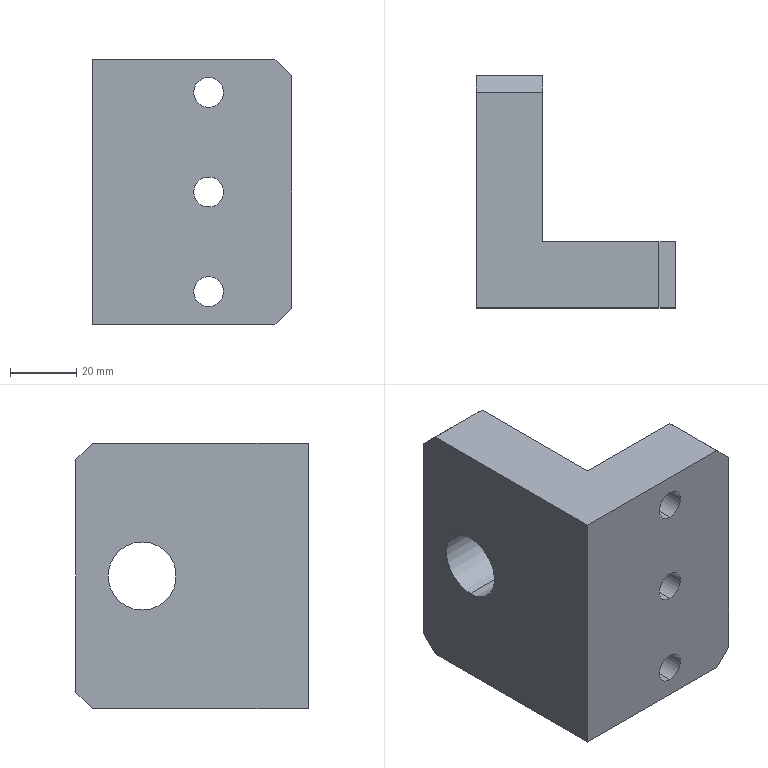Part | SolidWorks | features BaseBody 1 | 1 solid | 29 faces | box 60 x 70 x 80 mm | volume 161528 mm3 | plane 15 | cylinder 14 | commonest cylinder face diameters 9 x6 15 x6 20.5 x2
STEP:
#1=CARTESIAN_POINT('',(0.,50.,50.25));
#2=VERTEX_POINT('',#1);
#3=CARTESIAN_POINT('',(0.,50.,29.75));
#4=VERTEX_POINT('',#3);
#5=CARTESIAN_POINT('',(0.,50.,40.));
#6=DIRECTION('',(1.,0.,0.));
#7=DIRECTION('',(0.,0.,-1.));
#8=AXIS2_PLACEMENT_3D('',#5,#6,#7);
#9=CIRCLE('',#8,10.25);
#10=EDGE_CURVE('',#2,#4,#9,.T.);
#11=ORIENTED_EDGE('',*,*,#10,.F.);
#12=CARTESIAN_POINT('',(20.,50.,50.25));
#13=VERTEX_POINT('',#12);
#14=CARTESIAN_POINT('',(20.,50.,50.25));
#15=DIRECTION('',(1.,0.,0.));
#16=VECTOR('',#15,1000.);
#17=LINE('',#14,#16);
#18=EDGE_CURVE('',#2,#13,#17,.T.);
#19=ORIENTED_EDGE('',*,*,#18,.T.);
#20=CARTESIAN_POINT('',(20.,50.,29.75));
#21=VERTEX_POINT('',#20);
#22=CARTESIAN_POINT('',(20.,50.,40.));
#23=DIRECTION('',(1.,0.,0.));
#24=DIRECTION('',(0.,0.,-1.));
#25=AXIS2_PLACEMENT_3D('',#22,#23,#24);
#26=CIRCLE('',#25,10.25);
#27=EDGE_CURVE('',#13,#21,#26,.T.);
#28=ORIENTED_EDGE('',*,*,#27,.T.);
#29=CARTESIAN_POINT('',(20.,50.,29.75));
#30=DIRECTION('',(1.,0.,0.));
#31=VECTOR('',#30,1000.);
#32=LINE('',#29,#31);
#33=EDGE_CURVE('',#4,#21,#32,.T.);
#34=ORIENTED_EDGE('',*,*,#33,.F.);
#35=EDGE_LOOP('',(#11,#19,#28,#34));
#36=FACE_OUTER_BOUND('',#35,.T.);
#37=CARTESIAN_POINT('',(20.,50.,40.));
#38=DIRECTION('',(1.,0.,0.));
#39=DIRECTION('',(0.,0.,-1.));
#40=AXIS2_PLACEMENT_3D('',#37,#38,#39);
#41=CYLINDRICAL_SURFACE('',#40,10.25);
#42=ADVANCED_FACE('',(#36),#41,.F.);
#43=CARTESIAN_POINT('',(35.,11.,2.5));
#44=VERTEX_POINT('',#43);
#45=CARTESIAN_POINT('',(35.,11.,17.5));
#46=VERTEX_POINT('',#45);
#47=CARTESIAN_POINT('',(35.,11.,10.));
#48=DIRECTION('',(0.,1.,0.));
#49=DIRECTION('',(0.,0.,1.));
#50=AXIS2_PLACEMENT_3D('',#47,#48,#49);
#51=CIRCLE('',#50,7.5);
#52=EDGE_CURVE('',#44,#46,#51,.T.);
#53=ORIENTED_EDGE('',*,*,#52,.F.);
#54=CARTESIAN_POINT('',(35.,20.,2.5));
#55=VERTEX_POINT('',#54);
#56=CARTESIAN_POINT('',(35.,20.,2.5));
#57=DIRECTION('',(0.,1.,0.));
#58=VECTOR('',#57,1000.);
#59=LINE('',#56,#58);
#60=EDGE_CURVE('',#44,#55,#59,.T.);
#61=ORIENTED_EDGE('',*,*,#60,.T.);
#62=CARTESIAN_POINT('',(35.,20.,17.5));
#63=VERTEX_POINT('',#62);
#64=CARTESIAN_POINT('',(35.,20.,10.));
#65=DIRECTION('',(0.,1.,0.));
#66=DIRECTION('',(0.,0.,1.));
#67=AXIS2_PLACEMENT_3D('',#64,#65,#66);
#68=CIRCLE('',#67,7.5);
#69=EDGE_CURVE('',#55,#63,#68,.T.);
#70=ORIENTED_EDGE('',*,*,#69,.T.);
#71=CARTESIAN_POINT('',(35.,20.,17.5));
#72=DIRECTION('',(0.,1.,0.));
#73=VECTOR('',#72,1000.);
#74=LINE('',#71,#73);
#75=EDGE_CURVE('',#46,#63,#74,.T.);
#76=ORIENTED_EDGE('',*,*,#75,.F.);
#77=EDGE_LOOP('',(#53,#61,#70,#76));
#78=FACE_OUTER_BOUND('',#77,.T.);
#79=CARTESIAN_POINT('',(35.,20.,10.));
#80=DIRECTION('',(0.,1.,0.));
#81=DIRECTION('',(0.,0.,1.));
#82=AXIS2_PLACEMENT_3D('',#79,#80,#81);
#83=CYLINDRICAL_SURFACE('',#82,7.5);
#84=ADVANCED_FACE('',(#78),#83,.F.);
#85=CARTESIAN_POINT('',(35.,0.,5.5));
#86=VERTEX_POINT('',#85);
#87=CARTESIAN_POINT('',(35.,0.,14.5));
#88=VERTEX_POINT('',#87);
#89=CARTESIAN_POINT('',(35.,0.,10.));
#90=DIRECTION('',(0.,1.,0.));
#91=DIRECTION('',(0.,0.,1.));
#92=AXIS2_PLACEMENT_3D('',#89,#90,#91);
#93=CIRCLE('',#92,4.5);
#94=EDGE_CURVE('',#86,#88,#93,.T.);
#95=ORIENTED_EDGE('',*,*,#94,.F.);
#96=CARTESIAN_POINT('',(35.,11.,5.5));
#97=VERTEX_POINT('',#96);
#98=CARTESIAN_POINT('',(35.,20.,5.5));
#99=DIRECTION('',(0.,1.,0.));
#100=VECTOR('',#99,1000.);
#101=LINE('',#98,#100);
#102=EDGE_CURVE('',#86,#97,#101,.T.);
#103=ORIENTED_EDGE('',*,*,#102,.T.);
#104=CARTESIAN_POINT('',(35.,11.,14.5));
#105=VERTEX_POINT('',#104);
#106=CARTESIAN_POINT('',(35.,11.,10.));
#107=DIRECTION('',(0.,1.,0.));
#108=DIRECTION('',(0.,0.,1.));
#109=AXIS2_PLACEMENT_3D('',#106,#107,#108);
#110=CIRCLE('',#109,4.5);
#111=EDGE_CURVE('',#97,#105,#110,.T.);
#112=ORIENTED_EDGE('',*,*,#111,.T.);
#113=CARTESIAN_POINT('',(35.,20.,14.5));
#114=DIRECTION('',(0.,1.,0.));
#115=VECTOR('',#114,1000.);
#116=LINE('',#113,#115);
#117=EDGE_CURVE('',#88,#105,#116,.T.);
#118=ORIENTED_EDGE('',*,*,#117,.F.);
#119=EDGE_LOOP('',(#95,#103,#112,#118));
#120=FACE_OUTER_BOUND('',#119,.T.);
#121=CARTESIAN_POINT('',(35.,20.,10.));
#122=DIRECTION('',(0.,1.,0.));
#123=DIRECTION('',(0.,0.,1.));
#124=AXIS2_PLACEMENT_3D('',#121,#122,#123);
#125=CYLINDRICAL_SURFACE('',#124,4.5);
#126=ADVANCED_FACE('',(#120),#125,.F.);
#127=CARTESIAN_POINT('',(35.,11.,32.5));
#128=VERTEX_POINT('',#127);
#129=CARTESIAN_POINT('',(35.,11.,47.5));
#130=VERTEX_POINT('',#129);
#131=CARTESIAN_POINT('',(35.,11.,40.));
#132=DIRECTION('',(0.,1.,0.));
#133=DIRECTION('',(0.,0.,1.));
#134=AXIS2_PLACEMENT_3D('',#131,#132,#133);
#135=CIRCLE('',#134,7.5);
#136=EDGE_CURVE('',#128,#130,#135,.T.);
#137=ORIENTED_EDGE('',*,*,#136,.F.);
#138=CARTESIAN_POINT('',(35.,20.,32.5));
#139=VERTEX_POINT('',#138);
#140=CARTESIAN_POINT('',(35.,20.,32.5));
#141=DIRECTION('',(0.,1.,0.));
#142=VECTOR('',#141,1000.);
#143=LINE('',#140,#142);
#144=EDGE_CURVE('',#128,#139,#143,.T.);
#145=ORIENTED_EDGE('',*,*,#144,.T.);
#146=CARTESIAN_POINT('',(35.,20.,47.5));
#147=VERTEX_POINT('',#146);
#148=CARTESIAN_POINT('',(35.,20.,40.));
#149=DIRECTION('',(0.,1.,0.));
#150=DIRECTION('',(0.,0.,1.));
#151=AXIS2_PLACEMENT_3D('',#148,#149,#150);
#152=CIRCLE('',#151,7.5);
#153=EDGE_CURVE('',#139,#147,#152,.T.);
#154=ORIENTED_EDGE('',*,*,#153,.T.);
#155=CARTESIAN_POINT('',(35.,20.,47.5));
#156=DIRECTION('',(0.,1.,0.));
#157=VECTOR('',#156,1000.);
#158=LINE('',#155,#157);
#159=EDGE_CURVE('',#130,#147,#158,.T.);
#160=ORIENTED_EDGE('',*,*,#159,.F.);
#161=EDGE_LOOP('',(#137,#145,#154,#160));
#162=FACE_OUTER_BOUND('',#161,.T.);
#163=CARTESIAN_POINT('',(35.,20.,40.));
#164=DIRECTION('',(0.,1.,0.));
#165=DIRECTION('',(0.,0.,1.));
#166=AXIS2_PLACEMENT_3D('',#163,#164,#165);
#167=CYLINDRICAL_SURFACE('',#166,7.5);
#168=ADVANCED_FACE('',(#162),#167,.F.);
#169=CARTESIAN_POINT('',(35.,0.,35.5));
#170=VERTEX_POINT('',#169);
#171=CARTESIAN_POINT('',(35.,0.,44.5));
#172=VERTEX_POINT('',#171);
#173=CARTESIAN_POINT('',(35.,0.,40.));
#174=DIRECTION('',(0.,1.,0.));
#175=DIRECTION('',(0.,0.,1.));
#176=AXIS2_PLACEMENT_3D('',#173,#174,#175);
#177=CIRCLE('',#176,4.5);
#178=EDGE_CURVE('',#170,#172,#177,.T.);
#179=ORIENTED_EDGE('',*,*,#178,.F.);
#180=CARTESIAN_POINT('',(35.,11.,35.5));
#181=VERTEX_POINT('',#180);
#182=CARTESIAN_POINT('',(35.,20.,35.5));
#183=DIRECTION('',(0.,1.,0.));
#184=VECTOR('',#183,1000.);
#185=LINE('',#182,#184);
#186=EDGE_CURVE('',#170,#181,#185,.T.);
#187=ORIENTED_EDGE('',*,*,#186,.T.);
#188=CARTESIAN_POINT('',(35.,11.,44.5));
#189=VERTEX_POINT('',#188);
#190=CARTESIAN_POINT('',(35.,11.,40.));
#191=DIRECTION('',(0.,1.,0.));
#192=DIRECTION('',(0.,0.,1.));
#193=AXIS2_PLACEMENT_3D('',#190,#191,#192);
#194=CIRCLE('',#193,4.5);
#195=EDGE_CURVE('',#181,#189,#194,.T.);
#196=ORIENTED_EDGE('',*,*,#195,.T.);
#197=CARTESIAN_POINT('',(35.,20.,44.5));
#198=DIRECTION('',(0.,1.,0.));
#199=VECTOR('',#198,1000.);
#200=LINE('',#197,#199);
#201=EDGE_CURVE('',#172,#189,#200,.T.);
#202=ORIENTED_EDGE('',*,*,#201,.F.);
#203=EDGE_LOOP('',(#179,#187,#196,#202));
#204=FACE_OUTER_BOUND('',#203,.T.);
#205=CARTESIAN_POINT('',(35.,20.,40.));
#206=DIRECTION('',(0.,1.,0.));
#207=DIRECTION('',(0.,0.,1.));
#208=AXIS2_PLACEMENT_3D('',#205,#206,#207);
#209=CYLINDRICAL_SURFACE('',#208,4.5);
#210=ADVANCED_FACE('',(#204),#209,.F.);
#211=CARTESIAN_POINT('',(35.,11.,62.5));
#212=VERTEX_POINT('',#211);
#213=CARTESIAN_POINT('',(35.,11.,77.5));
#214=VERTEX_POINT('',#213);
#215=CARTESIAN_POINT('',(35.,11.,70.));
#216=DIRECTION('',(0.,1.,0.));
#217=DIRECTION('',(0.,0.,1.));
#218=AXIS2_PLACEMENT_3D('',#215,#216,#217);
#219=CIRCLE('',#218,7.5);
#220=EDGE_CURVE('',#212,#214,#219,.T.);
#221=ORIENTED_EDGE('',*,*,#220,.F.);
#222=CARTESIAN_POINT('',(35.,20.,62.5));
#223=VERTEX_POINT('',#222);
#224=CARTESIAN_POINT('',(35.,20.,62.5));
#225=DIRECTION('',(0.,1.,0.));
#226=VECTOR('',#225,1000.);
#227=LINE('',#224,#226);
#228=EDGE_CURVE('',#212,#223,#227,.T.);
#229=ORIENTED_EDGE('',*,*,#228,.T.);
#230=CARTESIAN_POINT('',(35.,20.,77.5));
#231=VERTEX_POINT('',#230);
#232=CARTESIAN_POINT('',(35.,20.,70.));
#233=DIRECTION('',(0.,1.,0.));
#234=DIRECTION('',(0.,0.,1.));
#235=AXIS2_PLACEMENT_3D('',#232,#233,#234);
#236=CIRCLE('',#235,7.5);
#237=EDGE_CURVE('',#223,#231,#236,.T.);
#238=ORIENTED_EDGE('',*,*,#237,.T.);
#239=CARTESIAN_POINT('',(35.,20.,77.5));
#240=DIRECTION('',(0.,1.,0.));
#241=VECTOR('',#240,1000.);
#242=LINE('',#239,#241);
#243=EDGE_CURVE('',#214,#231,#242,.T.);
#244=ORIENTED_EDGE('',*,*,#243,.F.);
#245=EDGE_LOOP('',(#221,#229,#238,#244));
#246=FACE_OUTER_BOUND('',#245,.T.);
#247=CARTESIAN_POINT('',(35.,20.,70.));
#248=DIRECTION('',(0.,1.,0.));
#249=DIRECTION('',(0.,0.,1.));
#250=AXIS2_PLACEMENT_3D('',#247,#248,#249);
#251=CYLINDRICAL_SURFACE('',#250,7.5);
#252=ADVANCED_FACE('',(#246),#251,.F.);
#253=CARTESIAN_POINT('',(35.,0.,65.5));
#254=VERTEX_POINT('',#253);
#255=CARTESIAN_POINT('',(35.,0.,74.5));
#256=VERTEX_POINT('',#255);
#257=CARTESIAN_POINT('',(35.,0.,70.));
#258=DIRECTION('',(0.,1.,0.));
#259=DIRECTION('',(0.,0.,1.));
#260=AXIS2_PLACEMENT_3D('',#257,#258,#259);
#261=CIRCLE('',#260,4.5);
#262=EDGE_CURVE('',#254,#256,#261,.T.);
#263=ORIENTED_EDGE('',*,*,#262,.F.);
#264=CARTESIAN_POINT('',(35.,11.,65.5));
#265=VERTEX_POINT('',#264);
#266=CARTESIAN_POINT('',(35.,20.,65.5));
#267=DIRECTION('',(0.,1.,0.));
#268=VECTOR('',#267,1000.);
#269=LINE('',#266,#268);
#270=EDGE_CURVE('',#254,#265,#269,.T.);
#271=ORIENTED_EDGE('',*,*,#270,.T.);
#272=CARTESIAN_POINT('',(35.,11.,74.5));
#273=VERTEX_POINT('',#272);
#274=CARTESIAN_POINT('',(35.,11.,70.));
#275=DIRECTION('',(0.,1.,0.));
#276=DIRECTION('',(0.,0.,1.));
#277=AXIS2_PLACEMENT_3D('',#274,#275,#276);
#278=CIRCLE('',#277,4.5);
#279=EDGE_CURVE('',#265,#273,#278,.T.);
#280=ORIENTED_EDGE('',*,*,#279,.T.);
#281=CARTESIAN_POINT('',(35.,20.,74.5));
#282=DIRECTION('',(0.,1.,0.));
#283=VECTOR('',#282,1000.);
#284=LINE('',#281,#283);
#285=EDGE_CURVE('',#256,#273,#284,.T.);
#286=ORIENTED_EDGE('',*,*,#285,.F.);
#287=EDGE_LOOP('',(#263,#271,#280,#286));
#288=FACE_OUTER_BOUND('',#287,.T.);
#289=CARTESIAN_POINT('',(35.,20.,70.));
#290=DIRECTION('',(0.,1.,0.));
#291=DIRECTION('',(0.,0.,1.));
#292=AXIS2_PLACEMENT_3D('',#289,#290,#291);
#293=CYLINDRICAL_SURFACE('',#292,4.5);
#294=ADVANCED_FACE('',(#288),#293,.F.);
#295=CARTESIAN_POINT('',(35.,0.,10.));
#296=DIRECTION('',(0.,1.,0.));
#297=DIRECTION('',(0.,0.,1.));
#298=AXIS2_PLACEMENT_3D('',#295,#296,#297);
#299=CIRCLE('',#298,4.5);
#300=EDGE_CURVE('',#88,#86,#299,.T.);
#301=ORIENTED_EDGE('',*,*,#300,.T.);
#302=ORIENTED_EDGE('',*,*,#94,.T.);
#303=EDGE_LOOP('',(#301,#302));
#304=FACE_BOUND('',#303,.T.);
#305=CARTESIAN_POINT('',(35.,0.,40.));
#306=DIRECTION('',(0.,1.,0.));
#307=DIRECTION('',(0.,0.,1.));
#308=AXIS2_PLACEMENT_3D('',#305,#306,#307);
#309=CIRCLE('',#308,4.5);
#310=EDGE_CURVE('',#172,#170,#309,.T.);
#311=ORIENTED_EDGE('',*,*,#310,.T.);
#312=ORIENTED_EDGE('',*,*,#178,.T.);
#313=EDGE_LOOP('',(#311,#312));
#314=FACE_BOUND('',#313,.T.);
#315=CARTESIAN_POINT('',(35.,0.,70.));
#316=DIRECTION('',(0.,1.,0.));
#317=DIRECTION('',(0.,0.,1.));
#318=AXIS2_PLACEMENT_3D('',#315,#316,#317);
#319=CIRCLE('',#318,4.5);
#320=EDGE_CURVE('',#256,#254,#319,.T.);
#321=ORIENTED_EDGE('',*,*,#320,.T.);
#322=ORIENTED_EDGE('',*,*,#262,.T.);
#323=EDGE_LOOP('',(#321,#322));
#324=FACE_BOUND('',#323,.T.);
#325=CARTESIAN_POINT('',(0.,0.,0.));
#326=VERTEX_POINT('',#325);
#327=CARTESIAN_POINT('',(55.,0.,0.));
#328=VERTEX_POINT('',#327);
#329=CARTESIAN_POINT('',(60.,0.,0.));
#330=DIRECTION('',(1.,0.,0.));
#331=VECTOR('',#330,1000.);
#332=LINE('',#329,#331);
#333=EDGE_CURVE('',#326,#328,#332,.T.);
#334=ORIENTED_EDGE('',*,*,#333,.T.);
#335=CARTESIAN_POINT('',(60.,0.,5.));
#336=VERTEX_POINT('',#335);
#337=CARTESIAN_POINT('',(60.,0.,5.));
#338=DIRECTION('',(0.7071,0.,0.7071));
#339=VECTOR('',#338,1000.);
#340=LINE('',#337,#339);
#341=EDGE_CURVE('',#328,#336,#340,.T.);
#342=ORIENTED_EDGE('',*,*,#341,.T.);
#343=CARTESIAN_POINT('',(60.,0.,75.));
#344=VERTEX_POINT('',#343);
#345=CARTESIAN_POINT('',(60.,0.,80.));
#346=DIRECTION('',(0.,0.,-1.));
#347=VECTOR('',#346,1000.);
#348=LINE('',#345,#347);
#349=EDGE_CURVE('',#344,#336,#348,.T.);
#350=ORIENTED_EDGE('',*,*,#349,.F.);
#351=CARTESIAN_POINT('',(55.,0.,80.));
#352=VERTEX_POINT('',#351);
#353=CARTESIAN_POINT('',(55.,0.,80.));
#354=DIRECTION('',(-0.7071,0.,0.7071));
#355=VECTOR('',#354,1000.);
#356=LINE('',#353,#355);
#357=EDGE_CURVE('',#344,#352,#356,.T.);
#358=ORIENTED_EDGE('',*,*,#357,.T.);
#359=CARTESIAN_POINT('',(0.,0.,80.));
#360=VERTEX_POINT('',#359);
#361=CARTESIAN_POINT('',(60.,0.,80.));
#362=DIRECTION('',(1.,0.,0.));
#363=VECTOR('',#362,1000.);
#364=LINE('',#361,#363);
#365=EDGE_CURVE('',#360,#352,#364,.T.);
#366=ORIENTED_EDGE('',*,*,#365,.F.);
#367=CARTESIAN_POINT('',(0.,0.,80.));
#368=DIRECTION('',(0.,0.,-1.));
#369=VECTOR('',#368,1000.);
#370=LINE('',#367,#369);
#371=EDGE_CURVE('',#360,#326,#370,.T.);
#372=ORIENTED_EDGE('',*,*,#371,.T.);
#373=EDGE_LOOP('',(#334,#342,#350,#358,#366,#372));
#374=FACE_OUTER_BOUND('',#373,.T.);
#375=CARTESIAN_POINT('',(60.,0.,80.));
#376=DIRECTION('',(0.,1.,0.));
#377=DIRECTION('',(-1.,0.,0.));
#378=AXIS2_PLACEMENT_3D('',#375,#376,#377);
#379=PLANE('',#378);
#380=ADVANCED_FACE('',(#304,#314,#324,#374),#379,.F.);
#381=ORIENTED_EDGE('',*,*,#349,.T.);
#382=CARTESIAN_POINT('',(60.,20.,5.));
#383=VERTEX_POINT('',#382);
#384=CARTESIAN_POINT('',(60.,20.,5.));
#385=DIRECTION('',(0.,1.,0.));
#386=VECTOR('',#385,1000.);
#387=LINE('',#384,#386);
#388=EDGE_CURVE('',#336,#383,#387,.T.);
#389=ORIENTED_EDGE('',*,*,#388,.T.);
#390=CARTESIAN_POINT('',(60.,20.,75.));
#391=VERTEX_POINT('',#390);
#392=CARTESIAN_POINT('',(60.,20.,80.));
#393=DIRECTION('',(0.,0.,-1.));
#394=VECTOR('',#393,1000.);
#395=LINE('',#392,#394);
#396=EDGE_CURVE('',#391,#383,#395,.T.);
#397=ORIENTED_EDGE('',*,*,#396,.F.);
#398=CARTESIAN_POINT('',(60.,20.,75.));
#399=DIRECTION('',(0.,-1.,0.));
#400=VECTOR('',#399,1000.);
#401=LINE('',#398,#400);
#402=EDGE_CURVE('',#391,#344,#401,.T.);
#403=ORIENTED_EDGE('',*,*,#402,.T.);
#404=EDGE_LOOP('',(#381,#389,#397,#403));
#405=FACE_OUTER_BOUND('',#404,.T.);
#406=CARTESIAN_POINT('',(60.,20.,80.));
#407=DIRECTION('',(-1.,0.,0.));
#408=DIRECTION('',(0.,0.,1.));
#409=AXIS2_PLACEMENT_3D('',#406,#407,#408);
#410=PLANE('',#409);
#411=ADVANCED_FACE('',(#405),#410,.F.);
#412=CARTESIAN_POINT('',(35.,20.,10.));
#413=DIRECTION('',(0.,1.,0.));
#414=DIRECTION('',(0.,0.,1.));
#415=AXIS2_PLACEMENT_3D('',#412,#413,#414);
#416=CIRCLE('',#415,7.5);
#417=EDGE_CURVE('',#63,#55,#416,.T.);
#418=ORIENTED_EDGE('',*,*,#417,.F.);
#419=ORIENTED_EDGE('',*,*,#69,.F.);
#420=EDGE_LOOP('',(#418,#419));
#421=FACE_BOUND('',#420,.T.);
#422=CARTESIAN_POINT('',(35.,20.,40.));
#423=DIRECTION('',(0.,1.,0.));
#424=DIRECTION('',(0.,0.,1.));
#425=AXIS2_PLACEMENT_3D('',#422,#423,#424);
#426=CIRCLE('',#425,7.5);
#427=EDGE_CURVE('',#147,#139,#426,.T.);
#428=ORIENTED_EDGE('',*,*,#427,.F.);
#429=ORIENTED_EDGE('',*,*,#153,.F.);
#430=EDGE_LOOP('',(#428,#429));
#431=FACE_BOUND('',#430,.T.);
#432=CARTESIAN_POINT('',(35.,20.,70.));
#433=DIRECTION('',(0.,1.,0.));
#434=DIRECTION('',(0.,0.,1.));
#435=AXIS2_PLACEMENT_3D('',#432,#433,#434);
#436=CIRCLE('',#435,7.5);
#437=EDGE_CURVE('',#231,#223,#436,.T.);
#438=ORIENTED_EDGE('',*,*,#437,.F.);
#439=ORIENTED_EDGE('',*,*,#237,.F.);
#440=EDGE_LOOP('',(#438,#439));
#441=FACE_BOUND('',#440,.T.);
#442=ORIENTED_EDGE('',*,*,#396,.T.);
#443=CARTESIAN_POINT('',(55.,20.,0.));
#444=VERTEX_POINT('',#443);
#445=CARTESIAN_POINT('',(60.,20.,5.));
#446=DIRECTION('',(-0.7071,0.,-0.7071));
#447=VECTOR('',#446,1000.);
#448=LINE('',#445,#447);
#449=EDGE_CURVE('',#383,#444,#448,.T.);
#450=ORIENTED_EDGE('',*,*,#449,.T.);
#451=CARTESIAN_POINT('',(20.,20.,0.));
#452=VERTEX_POINT('',#451);
#453=CARTESIAN_POINT('',(20.,20.,0.));
#454=DIRECTION('',(-1.,0.,0.));
#455=VECTOR('',#454,1000.);
#456=LINE('',#453,#455);
#457=EDGE_CURVE('',#444,#452,#456,.T.);
#458=ORIENTED_EDGE('',*,*,#457,.T.);
#459=CARTESIAN_POINT('',(20.,20.,80.));
#460=VERTEX_POINT('',#459);
#461=CARTESIAN_POINT('',(20.,20.,80.));
#462=DIRECTION('',(0.,0.,-1.));
#463=VECTOR('',#462,1000.);
#464=LINE('',#461,#463);
#465=EDGE_CURVE('',#460,#452,#464,.T.);
#466=ORIENTED_EDGE('',*,*,#465,.F.);
#467=CARTESIAN_POINT('',(55.,20.,80.));
#468=VERTEX_POINT('',#467);
#469=CARTESIAN_POINT('',(20.,20.,80.));
#470=DIRECTION('',(-1.,0.,0.));
#471=VECTOR('',#470,1000.);
#472=LINE('',#469,#471);
#473=EDGE_CURVE('',#468,#460,#472,.T.);
#474=ORIENTED_EDGE('',*,*,#473,.F.);
#475=CARTESIAN_POINT('',(55.,20.,80.));
#476=DIRECTION('',(0.7071,0.,-0.7071));
#477=VECTOR('',#476,1000.);
#478=LINE('',#475,#477);
#479=EDGE_CURVE('',#468,#391,#478,.T.);
#480=ORIENTED_EDGE('',*,*,#479,.T.);
#481=EDGE_LOOP('',(#442,#450,#458,#466,#474,#480));
#482=FACE_OUTER_BOUND('',#481,.T.);
#483=CARTESIAN_POINT('',(20.,20.,80.));
#484=DIRECTION('',(0.,-1.,0.));
#485=DIRECTION('',(0.,0.,-1.));
#486=AXIS2_PLACEMENT_3D('',#483,#484,#485);
#487=PLANE('',#486);
#488=ADVANCED_FACE('',(#421,#431,#441,#482),#487,.F.);
#489=CARTESIAN_POINT('',(20.,50.,40.));
#490=DIRECTION('',(1.,0.,0.));
#491=DIRECTION('',(0.,0.,-1.));
#492=AXIS2_PLACEMENT_3D('',#489,#490,#491);
#493=CIRCLE('',#492,10.25);
#494=EDGE_CURVE('',#21,#13,#493,.T.);
#495=ORIENTED_EDGE('',*,*,#494,.F.);
#496=ORIENTED_EDGE('',*,*,#27,.F.);
#497=EDGE_LOOP('',(#495,#496));
#498=FACE_BOUND('',#497,.T.);
#499=CARTESIAN_POINT('',(20.,70.,75.));
#500=VERTEX_POINT('',#499);
#501=CARTESIAN_POINT('',(20.,70.,5.));
#502=VERTEX_POINT('',#501);
#503=CARTESIAN_POINT('',(20.,70.,80.));
#504=DIRECTION('',(0.,0.,-1.));
#505=VECTOR('',#504,1000.);
#506=LINE('',#503,#505);
#507=EDGE_CURVE('',#500,#502,#506,.T.);
#508=ORIENTED_EDGE('',*,*,#507,.F.);
#509=CARTESIAN_POINT('',(20.,65.,80.));
#510=VERTEX_POINT('',#509);
#511=CARTESIAN_POINT('',(20.,65.,80.));
#512=DIRECTION('',(0.,-0.7071,0.7071));
#513=VECTOR('',#512,1000.);
#514=LINE('',#511,#513);
#515=EDGE_CURVE('',#500,#510,#514,.T.);
#516=ORIENTED_EDGE('',*,*,#515,.T.);
#517=CARTESIAN_POINT('',(20.,70.,80.));
#518=DIRECTION('',(0.,1.,0.));
#519=VECTOR('',#518,1000.);
#520=LINE('',#517,#519);
#521=EDGE_CURVE('',#460,#510,#520,.T.);
#522=ORIENTED_EDGE('',*,*,#521,.F.);
#523=ORIENTED_EDGE('',*,*,#465,.T.);
#524=CARTESIAN_POINT('',(20.,65.,0.));
#525=VERTEX_POINT('',#524);
#526=CARTESIAN_POINT('',(20.,70.,0.));
#527=DIRECTION('',(0.,1.,0.));
#528=VECTOR('',#527,1000.);
#529=LINE('',#526,#528);
#530=EDGE_CURVE('',#452,#525,#529,.T.);
#531=ORIENTED_EDGE('',*,*,#530,.T.);
#532=CARTESIAN_POINT('',(20.,70.,5.));
#533=DIRECTION('',(0.,0.7071,0.7071));
#534=VECTOR('',#533,1000.);
#535=LINE('',#532,#534);
#536=EDGE_CURVE('',#525,#502,#535,.T.);
#537=ORIENTED_EDGE('',*,*,#536,.T.);
#538=EDGE_LOOP('',(#508,#516,#522,#523,#531,#537));
#539=FACE_OUTER_BOUND('',#538,.T.);
#540=CARTESIAN_POINT('',(20.,70.,80.));
#541=DIRECTION('',(-1.,0.,0.));
#542=DIRECTION('',(0.,-1.,0.));
#543=AXIS2_PLACEMENT_3D('',#540,#541,#542);
#544=PLANE('',#543);
#545=ADVANCED_FACE('',(#498,#539),#544,.F.);
#546=CARTESIAN_POINT('',(0.,70.,75.));
#547=VERTEX_POINT('',#546);
#548=CARTESIAN_POINT('',(0.,70.,5.));
#549=VERTEX_POINT('',#548);
#550=CARTESIAN_POINT('',(0.,70.,80.));
#551=DIRECTION('',(0.,0.,-1.));
#552=VECTOR('',#551,1000.);
#553=LINE('',#550,#552);
#554=EDGE_CURVE('',#547,#549,#553,.T.);
#555=ORIENTED_EDGE('',*,*,#554,.F.);
#556=CARTESIAN_POINT('',(0.,70.,75.));
#557=DIRECTION('',(1.,0.,0.));
#558=VECTOR('',#557,1000.);
#559=LINE('',#556,#558);
#560=EDGE_CURVE('',#547,#500,#559,.T.);
#561=ORIENTED_EDGE('',*,*,#560,.T.);
#562=ORIENTED_EDGE('',*,*,#507,.T.);
#563=CARTESIAN_POINT('',(0.,70.,5.));
#564=DIRECTION('',(-1.,0.,0.));
#565=VECTOR('',#564,1000.);
#566=LINE('',#563,#565);
#567=EDGE_CURVE('',#502,#549,#566,.T.);
#568=ORIENTED_EDGE('',*,*,#567,.T.);
#569=EDGE_LOOP('',(#555,#561,#562,#568));
#570=FACE_OUTER_BOUND('',#569,.T.);
#571=CARTESIAN_POINT('',(0.,70.,80.));
#572=DIRECTION('',(0.,-1.,0.));
#573=DIRECTION('',(0.,0.,-1.));
#574=AXIS2_PLACEMENT_3D('',#571,#572,#573);
#575=PLANE('',#574);
#576=ADVANCED_FACE('',(#570),#575,.F.);
#577=CARTESIAN_POINT('',(0.,50.,40.));
#578=DIRECTION('',(1.,0.,0.));
#579=DIRECTION('',(0.,0.,-1.));
#580=AXIS2_PLACEMENT_3D('',#577,#578,#579);
#581=CIRCLE('',#580,10.25);
#582=EDGE_CURVE('',#4,#2,#581,.T.);
#583=ORIENTED_EDGE('',*,*,#582,.T.);
#584=ORIENTED_EDGE('',*,*,#10,.T.);
#585=EDGE_LOOP('',(#583,#584));
#586=FACE_BOUND('',#585,.T.);
#587=CARTESIAN_POINT('',(0.,65.,80.));
#588=VERTEX_POINT('',#587);
#589=CARTESIAN_POINT('',(0.,0.,80.));
#590=DIRECTION('',(0.,-1.,0.));
#591=VECTOR('',#590,1000.);
#592=LINE('',#589,#591);
#593=EDGE_CURVE('',#588,#360,#592,.T.);
#594=ORIENTED_EDGE('',*,*,#593,.F.);
#595=CARTESIAN_POINT('',(0.,65.,80.));
#596=DIRECTION('',(0.,0.7071,-0.7071));
#597=VECTOR('',#596,1000.);
#598=LINE('',#595,#597);
#599=EDGE_CURVE('',#588,#547,#598,.T.);
#600=ORIENTED_EDGE('',*,*,#599,.T.);
#601=ORIENTED_EDGE('',*,*,#554,.T.);
#602=CARTESIAN_POINT('',(0.,65.,0.));
#603=VERTEX_POINT('',#602);
#604=CARTESIAN_POINT('',(0.,70.,5.));
#605=DIRECTION('',(0.,-0.7071,-0.7071));
#606=VECTOR('',#605,1000.);
#607=LINE('',#604,#606);
#608=EDGE_CURVE('',#549,#603,#607,.T.);
#609=ORIENTED_EDGE('',*,*,#608,.T.);
#610=CARTESIAN_POINT('',(0.,0.,0.));
#611=DIRECTION('',(0.,-1.,0.));
#612=VECTOR('',#611,1000.);
#613=LINE('',#610,#612);
#614=EDGE_CURVE('',#603,#326,#613,.T.);
#615=ORIENTED_EDGE('',*,*,#614,.T.);
#616=ORIENTED_EDGE('',*,*,#371,.F.);
#617=EDGE_LOOP('',(#594,#600,#601,#609,#615,#616));
#618=FACE_OUTER_BOUND('',#617,.T.);
#619=CARTESIAN_POINT('',(0.,0.,80.));
#620=DIRECTION('',(1.,0.,0.));
#621=DIRECTION('',(0.,0.,-1.));
#622=AXIS2_PLACEMENT_3D('',#619,#620,#621);
#623=PLANE('',#622);
#624=ADVANCED_FACE('',(#586,#618),#623,.F.);
#625=ORIENTED_EDGE('',*,*,#521,.T.);
#626=CARTESIAN_POINT('',(0.,65.,80.));
#627=DIRECTION('',(-1.,0.,0.));
#628=VECTOR('',#627,1000.);
#629=LINE('',#626,#628);
#630=EDGE_CURVE('',#510,#588,#629,.T.);
#631=ORIENTED_EDGE('',*,*,#630,.T.);
#632=ORIENTED_EDGE('',*,*,#593,.T.);
#633=ORIENTED_EDGE('',*,*,#365,.T.);
#634=CARTESIAN_POINT('',(55.,0.,80.));
#635=DIRECTION('',(0.,1.,0.));
#636=VECTOR('',#635,1000.);
#637=LINE('',#634,#636);
#638=EDGE_CURVE('',#352,#468,#637,.T.);
#639=ORIENTED_EDGE('',*,*,#638,.T.);
#640=ORIENTED_EDGE('',*,*,#473,.T.);
#641=EDGE_LOOP('',(#625,#631,#632,#633,#639,#640));
#642=FACE_OUTER_BOUND('',#641,.T.);
#643=CARTESIAN_POINT('',(0.,0.,80.));
#644=DIRECTION('',(0.,0.,-1.));
#645=DIRECTION('',(-1.,0.,0.));
#646=AXIS2_PLACEMENT_3D('',#643,#644,#645);
#647=PLANE('',#646);
#648=ADVANCED_FACE('',(#642),#647,.F.);
#649=ORIENTED_EDGE('',*,*,#614,.F.);
#650=CARTESIAN_POINT('',(20.,65.,0.));
#651=DIRECTION('',(1.,0.,0.));
#652=VECTOR('',#651,1000.);
#653=LINE('',#650,#652);
#654=EDGE_CURVE('',#603,#525,#653,.T.);
#655=ORIENTED_EDGE('',*,*,#654,.T.);
#656=ORIENTED_EDGE('',*,*,#530,.F.);
#657=ORIENTED_EDGE('',*,*,#457,.F.);
#658=CARTESIAN_POINT('',(55.,0.,0.));
#659=DIRECTION('',(0.,-1.,0.));
#660=VECTOR('',#659,1000.);
#661=LINE('',#658,#660);
#662=EDGE_CURVE('',#444,#328,#661,.T.);
#663=ORIENTED_EDGE('',*,*,#662,.T.);
#664=ORIENTED_EDGE('',*,*,#333,.F.);
#665=EDGE_LOOP('',(#649,#655,#656,#657,#663,#664));
#666=FACE_OUTER_BOUND('',#665,.T.);
#667=CARTESIAN_POINT('',(0.,0.,0.));
#668=DIRECTION('',(0.,0.,-1.));
#669=DIRECTION('',(-1.,0.,0.));
#670=AXIS2_PLACEMENT_3D('',#667,#668,#669);
#671=PLANE('',#670);
#672=ADVANCED_FACE('',(#666),#671,.T.);
#673=ORIENTED_EDGE('',*,*,#270,.F.);
#674=ORIENTED_EDGE('',*,*,#320,.F.);
#675=ORIENTED_EDGE('',*,*,#285,.T.);
#676=CARTESIAN_POINT('',(35.,11.,70.));
#677=DIRECTION('',(0.,1.,0.));
#678=DIRECTION('',(0.,0.,1.));
#679=AXIS2_PLACEMENT_3D('',#676,#677,#678);
#680=CIRCLE('',#679,4.5);
#681=EDGE_CURVE('',#273,#265,#680,.T.);
#682=ORIENTED_EDGE('',*,*,#681,.T.);
#683=EDGE_LOOP('',(#673,#674,#675,#682));
#684=FACE_OUTER_BOUND('',#683,.T.);
#685=CARTESIAN_POINT('',(35.,20.,70.));
#686=DIRECTION('',(0.,1.,0.));
#687=DIRECTION('',(0.,0.,1.));
#688=AXIS2_PLACEMENT_3D('',#685,#686,#687);
#689=CYLINDRICAL_SURFACE('',#688,4.5);
#690=ADVANCED_FACE('',(#684),#689,.F.);
#691=ORIENTED_EDGE('',*,*,#681,.F.);
#692=ORIENTED_EDGE('',*,*,#279,.F.);
#693=EDGE_LOOP('',(#691,#692));
#694=FACE_BOUND('',#693,.T.);
#695=CARTESIAN_POINT('',(35.,11.,70.));
#696=DIRECTION('',(0.,1.,0.));
#697=DIRECTION('',(0.,0.,1.));
#698=AXIS2_PLACEMENT_3D('',#695,#696,#697);
#699=CIRCLE('',#698,7.5);
#700=EDGE_CURVE('',#214,#212,#699,.T.);
#701=ORIENTED_EDGE('',*,*,#700,.T.);
#702=ORIENTED_EDGE('',*,*,#220,.T.);
#703=EDGE_LOOP('',(#701,#702));
#704=FACE_OUTER_BOUND('',#703,.T.);
#705=CARTESIAN_POINT('',(39.5,11.,70.));
#706=DIRECTION('',(0.,-1.,0.));
#707=DIRECTION('',(0.,0.,-1.));
#708=AXIS2_PLACEMENT_3D('',#705,#706,#707);
#709=PLANE('',#708);
#710=ADVANCED_FACE('',(#694,#704),#709,.F.);
#711=ORIENTED_EDGE('',*,*,#228,.F.);
#712=ORIENTED_EDGE('',*,*,#700,.F.);
#713=ORIENTED_EDGE('',*,*,#243,.T.);
#714=ORIENTED_EDGE('',*,*,#437,.T.);
#715=EDGE_LOOP('',(#711,#712,#713,#714));
#716=FACE_OUTER_BOUND('',#715,.T.);
#717=CARTESIAN_POINT('',(35.,20.,70.));
#718=DIRECTION('',(0.,1.,0.));
#719=DIRECTION('',(0.,0.,1.));
#720=AXIS2_PLACEMENT_3D('',#717,#718,#719);
#721=CYLINDRICAL_SURFACE('',#720,7.5);
#722=ADVANCED_FACE('',(#716),#721,.F.);
#723=ORIENTED_EDGE('',*,*,#186,.F.);
#724=ORIENTED_EDGE('',*,*,#310,.F.);
#725=ORIENTED_EDGE('',*,*,#201,.T.);
#726=CARTESIAN_POINT('',(35.,11.,40.));
#727=DIRECTION('',(0.,1.,0.));
#728=DIRECTION('',(0.,0.,1.));
#729=AXIS2_PLACEMENT_3D('',#726,#727,#728);
#730=CIRCLE('',#729,4.5);
#731=EDGE_CURVE('',#189,#181,#730,.T.);
#732=ORIENTED_EDGE('',*,*,#731,.T.);
#733=EDGE_LOOP('',(#723,#724,#725,#732));
#734=FACE_OUTER_BOUND('',#733,.T.);
#735=CARTESIAN_POINT('',(35.,20.,40.));
#736=DIRECTION('',(0.,1.,0.));
#737=DIRECTION('',(0.,0.,1.));
#738=AXIS2_PLACEMENT_3D('',#735,#736,#737);
#739=CYLINDRICAL_SURFACE('',#738,4.5);
#740=ADVANCED_FACE('',(#734),#739,.F.);
#741=ORIENTED_EDGE('',*,*,#731,.F.);
#742=ORIENTED_EDGE('',*,*,#195,.F.);
#743=EDGE_LOOP('',(#741,#742));
#744=FACE_BOUND('',#743,.T.);
#745=CARTESIAN_POINT('',(35.,11.,40.));
#746=DIRECTION('',(0.,1.,0.));
#747=DIRECTION('',(0.,0.,1.));
#748=AXIS2_PLACEMENT_3D('',#745,#746,#747);
#749=CIRCLE('',#748,7.5);
#750=EDGE_CURVE('',#130,#128,#749,.T.);
#751=ORIENTED_EDGE('',*,*,#750,.T.);
#752=ORIENTED_EDGE('',*,*,#136,.T.);
#753=EDGE_LOOP('',(#751,#752));
#754=FACE_OUTER_BOUND('',#753,.T.);
#755=CARTESIAN_POINT('',(39.5,11.,40.));
#756=DIRECTION('',(0.,-1.,0.));
#757=DIRECTION('',(0.,0.,-1.));
#758=AXIS2_PLACEMENT_3D('',#755,#756,#757);
#759=PLANE('',#758);
#760=ADVANCED_FACE('',(#744,#754),#759,.F.);
#761=ORIENTED_EDGE('',*,*,#144,.F.);
#762=ORIENTED_EDGE('',*,*,#750,.F.);
#763=ORIENTED_EDGE('',*,*,#159,.T.);
#764=ORIENTED_EDGE('',*,*,#427,.T.);
#765=EDGE_LOOP('',(#761,#762,#763,#764));
#766=FACE_OUTER_BOUND('',#765,.T.);
#767=CARTESIAN_POINT('',(35.,20.,40.));
#768=DIRECTION('',(0.,1.,0.));
#769=DIRECTION('',(0.,0.,1.));
#770=AXIS2_PLACEMENT_3D('',#767,#768,#769);
#771=CYLINDRICAL_SURFACE('',#770,7.5);
#772=ADVANCED_FACE('',(#766),#771,.F.);
#773=ORIENTED_EDGE('',*,*,#102,.F.);
#774=ORIENTED_EDGE('',*,*,#300,.F.);
#775=ORIENTED_EDGE('',*,*,#117,.T.);
#776=CARTESIAN_POINT('',(35.,11.,10.));
#777=DIRECTION('',(0.,1.,0.));
#778=DIRECTION('',(0.,0.,1.));
#779=AXIS2_PLACEMENT_3D('',#776,#777,#778);
#780=CIRCLE('',#779,4.5);
#781=EDGE_CURVE('',#105,#97,#780,.T.);
#782=ORIENTED_EDGE('',*,*,#781,.T.);
#783=EDGE_LOOP('',(#773,#774,#775,#782));
#784=FACE_OUTER_BOUND('',#783,.T.);
#785=CARTESIAN_POINT('',(35.,20.,10.));
#786=DIRECTION('',(0.,1.,0.));
#787=DIRECTION('',(0.,0.,1.));
#788=AXIS2_PLACEMENT_3D('',#785,#786,#787);
#789=CYLINDRICAL_SURFACE('',#788,4.5);
#790=ADVANCED_FACE('',(#784),#789,.F.);
#791=ORIENTED_EDGE('',*,*,#781,.F.);
#792=ORIENTED_EDGE('',*,*,#111,.F.);
#793=EDGE_LOOP('',(#791,#792));
#794=FACE_BOUND('',#793,.T.);
#795=CARTESIAN_POINT('',(35.,11.,10.));
#796=DIRECTION('',(0.,1.,0.));
#797=DIRECTION('',(0.,0.,1.));
#798=AXIS2_PLACEMENT_3D('',#795,#796,#797);
#799=CIRCLE('',#798,7.5);
#800=EDGE_CURVE('',#46,#44,#799,.T.);
#801=ORIENTED_EDGE('',*,*,#800,.T.);
#802=ORIENTED_EDGE('',*,*,#52,.T.);
#803=EDGE_LOOP('',(#801,#802));
#804=FACE_OUTER_BOUND('',#803,.T.);
#805=CARTESIAN_POINT('',(39.5,11.,10.));
#806=DIRECTION('',(0.,-1.,0.));
#807=DIRECTION('',(0.,0.,-1.));
#808=AXIS2_PLACEMENT_3D('',#805,#806,#807);
#809=PLANE('',#808);
#810=ADVANCED_FACE('',(#794,#804),#809,.F.);
#811=ORIENTED_EDGE('',*,*,#60,.F.);
#812=ORIENTED_EDGE('',*,*,#800,.F.);
#813=ORIENTED_EDGE('',*,*,#75,.T.);
#814=ORIENTED_EDGE('',*,*,#417,.T.);
#815=EDGE_LOOP('',(#811,#812,#813,#814));
#816=FACE_OUTER_BOUND('',#815,.T.);
#817=CARTESIAN_POINT('',(35.,20.,10.));
#818=DIRECTION('',(0.,1.,0.));
#819=DIRECTION('',(0.,0.,1.));
#820=AXIS2_PLACEMENT_3D('',#817,#818,#819);
#821=CYLINDRICAL_SURFACE('',#820,7.5);
#822=ADVANCED_FACE('',(#816),#821,.F.);
#823=ORIENTED_EDGE('',*,*,#515,.F.);
#824=ORIENTED_EDGE('',*,*,#560,.F.);
#825=ORIENTED_EDGE('',*,*,#599,.F.);
#826=ORIENTED_EDGE('',*,*,#630,.F.);
#827=EDGE_LOOP('',(#823,#824,#825,#826));
#828=FACE_OUTER_BOUND('',#827,.T.);
#829=CARTESIAN_POINT('',(0.,65.,80.));
#830=DIRECTION('',(0.,-0.7071,-0.7071));
#831=DIRECTION('',(-1.,0.,0.));
#832=AXIS2_PLACEMENT_3D('',#829,#830,#831);
#833=PLANE('',#832);
#834=ADVANCED_FACE('',(#828),#833,.F.);
#835=ORIENTED_EDGE('',*,*,#536,.F.);
#836=ORIENTED_EDGE('',*,*,#654,.F.);
#837=ORIENTED_EDGE('',*,*,#608,.F.);
#838=ORIENTED_EDGE('',*,*,#567,.F.);
#839=EDGE_LOOP('',(#835,#836,#837,#838));
#840=FACE_OUTER_BOUND('',#839,.T.);
#841=CARTESIAN_POINT('',(0.,70.,5.));
#842=DIRECTION('',(0.,0.7071,-0.7071));
#843=DIRECTION('',(1.,0.,0.));
#844=AXIS2_PLACEMENT_3D('',#841,#842,#843);
#845=PLANE('',#844);
#846=ADVANCED_FACE('',(#840),#845,.T.);
#847=ORIENTED_EDGE('',*,*,#341,.F.);
#848=ORIENTED_EDGE('',*,*,#662,.F.);
#849=ORIENTED_EDGE('',*,*,#449,.F.);
#850=ORIENTED_EDGE('',*,*,#388,.F.);
#851=EDGE_LOOP('',(#847,#848,#849,#850));
#852=FACE_OUTER_BOUND('',#851,.T.);
#853=CARTESIAN_POINT('',(60.,20.,5.));
#854=DIRECTION('',(0.7071,0.,-0.7071));
#855=DIRECTION('',(0.,-1.,0.));
#856=AXIS2_PLACEMENT_3D('',#853,#854,#855);
#857=PLANE('',#856);
#858=ADVANCED_FACE('',(#852),#857,.T.);
#859=ORIENTED_EDGE('',*,*,#357,.F.);
#860=ORIENTED_EDGE('',*,*,#402,.F.);
#861=ORIENTED_EDGE('',*,*,#479,.F.);
#862=ORIENTED_EDGE('',*,*,#638,.F.);
#863=EDGE_LOOP('',(#859,#860,#861,#862));
#864=FACE_OUTER_BOUND('',#863,.T.);
#865=CARTESIAN_POINT('',(55.,0.,80.));
#866=DIRECTION('',(-0.7071,0.,-0.7071));
#867=DIRECTION('',(0.,1.,0.));
#868=AXIS2_PLACEMENT_3D('',#865,#866,#867);
#869=PLANE('',#868);
#870=ADVANCED_FACE('',(#864),#869,.F.);
#871=ORIENTED_EDGE('',*,*,#18,.F.);
#872=ORIENTED_EDGE('',*,*,#582,.F.);
#873=ORIENTED_EDGE('',*,*,#33,.T.);
#874=ORIENTED_EDGE('',*,*,#494,.T.);
#875=EDGE_LOOP('',(#871,#872,#873,#874));
#876=FACE_OUTER_BOUND('',#875,.T.);
#877=CARTESIAN_POINT('',(20.,50.,40.));
#878=DIRECTION('',(1.,0.,0.));
#879=DIRECTION('',(0.,0.,-1.));
#880=AXIS2_PLACEMENT_3D('',#877,#878,#879);
#881=CYLINDRICAL_SURFACE('',#880,10.25);
#882=ADVANCED_FACE('',(#876),#881,.F.);
#883=CLOSED_SHELL('',(#42,#84,#126,#168,#210,#252,#294,#380,#411,#488,#545,#576,#624,#648,#672,#690,#710,#722,#740,#760,#772,#790,#810,#822,#834,#846,#858,#870,#882));
#884=MANIFOLD_SOLID_BREP('',#883);
#885=CARTESIAN_POINT('',(0.,0.,0.));
#886=DIRECTION('',(0.,0.,1.));
#887=DIRECTION('',(1.,0.,0.));
#888=AXIS2_PLACEMENT_3D('',#885,#886,#887);
#889=(LENGTH_UNIT()NAMED_UNIT(*)SI_UNIT(.MILLI.,.METRE.));
#890=UNCERTAINTY_MEASURE_WITH_UNIT(LENGTH_MEASURE(0.00001),#889,'','');
#891=(NAMED_UNIT(*)PLANE_ANGLE_UNIT()SI_UNIT($,.RADIAN.));
#892=(NAMED_UNIT(*)SI_UNIT($,.STERADIAN.)SOLID_ANGLE_UNIT());
#893=(GEOMETRIC_REPRESENTATION_CONTEXT(3)GLOBAL_UNCERTAINTY_ASSIGNED_CONTEXT((#890))GLOBAL_UNIT_ASSIGNED_CONTEXT((#889,#891,#892))REPRESENTATION_CONTEXT('',''));
#894=ADVANCED_BREP_SHAPE_REPRESENTATION('',(#884,#888),#893);